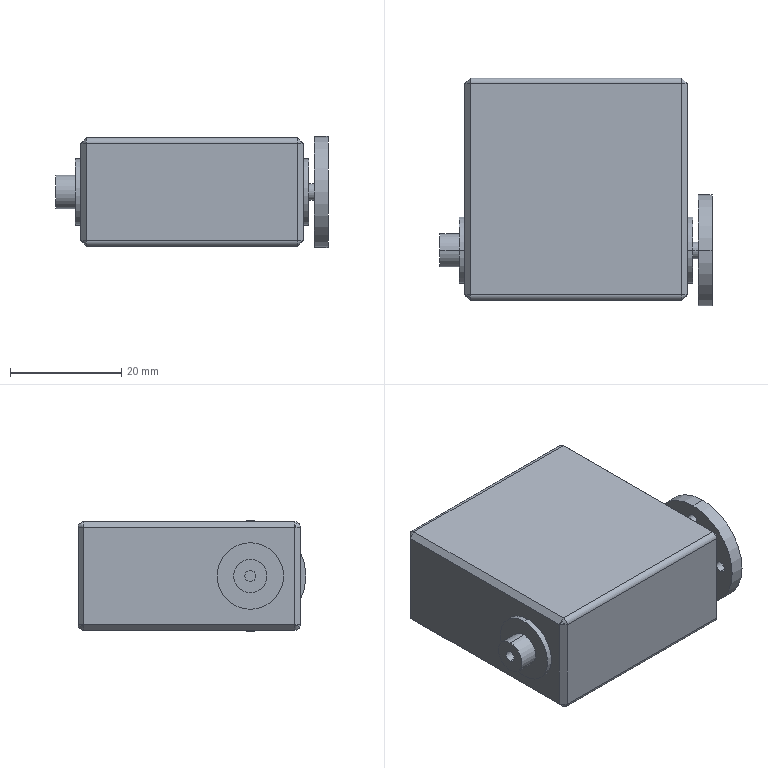Part | SolidWorks | features ICE 7, Chamfer 1, Extrusion 1, Fillet 1 | 1 solid | 52 faces | box 49 x 41 x 20 mm | volume 32126 mm3 | cylinder 24 | plane 20 | cone 8 | commonest cylinder face diameters 2 x14 12 x4 3 x2 6 x2 20 x2
STEP:
#1=CARTESIAN_POINT('',(42.,16.,8.75));
#2=VERTEX_POINT('',#1);
#3=CARTESIAN_POINT('',(42.,16.,10.75));
#4=VERTEX_POINT('',#3);
#5=CARTESIAN_POINT('',(42.,16.,9.75));
#6=DIRECTION('',(-1.,0.,0.));
#7=DIRECTION('',(0.,0.,-1.));
#8=AXIS2_PLACEMENT_3D('',#5,#6,#7);
#9=CIRCLE('',#8,1.);
#10=EDGE_CURVE('',#2,#4,#9,.T.);
#11=ORIENTED_EDGE('',*,*,#10,.T.);
#12=CARTESIAN_POINT('',(44.5,16.,10.75));
#13=VERTEX_POINT('',#12);
#14=CARTESIAN_POINT('',(-4.501,16.,10.75));
#15=DIRECTION('',(1.,0.,0.));
#16=VECTOR('',#15,1000.);
#17=LINE('',#14,#16);
#18=EDGE_CURVE('',#4,#13,#17,.T.);
#19=ORIENTED_EDGE('',*,*,#18,.T.);
#20=CARTESIAN_POINT('',(44.5,16.,8.75));
#21=VERTEX_POINT('',#20);
#22=CARTESIAN_POINT('',(44.5,16.,9.75));
#23=DIRECTION('',(1.,0.,0.));
#24=DIRECTION('',(0.,0.,-1.));
#25=AXIS2_PLACEMENT_3D('',#22,#23,#24);
#26=CIRCLE('',#25,1.);
#27=EDGE_CURVE('',#13,#21,#26,.T.);
#28=ORIENTED_EDGE('',*,*,#27,.T.);
#29=CARTESIAN_POINT('',(-4.501,16.,8.75));
#30=DIRECTION('',(1.,0.,0.));
#31=VECTOR('',#30,1000.);
#32=LINE('',#29,#31);
#33=EDGE_CURVE('',#2,#21,#32,.T.);
#34=ORIENTED_EDGE('',*,*,#33,.F.);
#35=EDGE_LOOP('',(#11,#19,#28,#34));
#36=FACE_OUTER_BOUND('',#35,.T.);
#37=CARTESIAN_POINT('',(-4.501,16.,9.75));
#38=DIRECTION('',(1.,0.,0.));
#39=DIRECTION('',(0.,0.,-1.));
#40=AXIS2_PLACEMENT_3D('',#37,#38,#39);
#41=CYLINDRICAL_SURFACE('',#40,1.);
#42=ADVANCED_FACE('',(#36),#41,.F.);
#43=CARTESIAN_POINT('',(42.,9.,15.75));
#44=VERTEX_POINT('',#43);
#45=CARTESIAN_POINT('',(42.,9.,17.75));
#46=VERTEX_POINT('',#45);
#47=CARTESIAN_POINT('',(42.,9.,16.75));
#48=DIRECTION('',(-1.,0.,0.));
#49=DIRECTION('',(0.,0.,-1.));
#50=AXIS2_PLACEMENT_3D('',#47,#48,#49);
#51=CIRCLE('',#50,1.);
#52=EDGE_CURVE('',#44,#46,#51,.T.);
#53=ORIENTED_EDGE('',*,*,#52,.T.);
#54=CARTESIAN_POINT('',(44.5,9.,17.75));
#55=VERTEX_POINT('',#54);
#56=CARTESIAN_POINT('',(-4.501,9.,17.75));
#57=DIRECTION('',(1.,0.,0.));
#58=VECTOR('',#57,1000.);
#59=LINE('',#56,#58);
#60=EDGE_CURVE('',#46,#55,#59,.T.);
#61=ORIENTED_EDGE('',*,*,#60,.T.);
#62=CARTESIAN_POINT('',(44.5,9.,15.75));
#63=VERTEX_POINT('',#62);
#64=CARTESIAN_POINT('',(44.5,9.,16.75));
#65=DIRECTION('',(1.,0.,0.));
#66=DIRECTION('',(0.,0.,-1.));
#67=AXIS2_PLACEMENT_3D('',#64,#65,#66);
#68=CIRCLE('',#67,1.);
#69=EDGE_CURVE('',#55,#63,#68,.T.);
#70=ORIENTED_EDGE('',*,*,#69,.T.);
#71=CARTESIAN_POINT('',(-4.501,9.,15.75));
#72=DIRECTION('',(1.,0.,0.));
#73=VECTOR('',#72,1000.);
#74=LINE('',#71,#73);
#75=EDGE_CURVE('',#44,#63,#74,.T.);
#76=ORIENTED_EDGE('',*,*,#75,.F.);
#77=EDGE_LOOP('',(#53,#61,#70,#76));
#78=FACE_OUTER_BOUND('',#77,.T.);
#79=CARTESIAN_POINT('',(-4.501,9.,16.75));
#80=DIRECTION('',(1.,0.,0.));
#81=DIRECTION('',(0.,0.,-1.));
#82=AXIS2_PLACEMENT_3D('',#79,#80,#81);
#83=CYLINDRICAL_SURFACE('',#82,1.);
#84=ADVANCED_FACE('',(#78),#83,.F.);
#85=CARTESIAN_POINT('',(42.,9.,1.75));
#86=VERTEX_POINT('',#85);
#87=CARTESIAN_POINT('',(42.,9.,3.75));
#88=VERTEX_POINT('',#87);
#89=CARTESIAN_POINT('',(42.,9.,2.75));
#90=DIRECTION('',(-1.,0.,0.));
#91=DIRECTION('',(0.,0.,-1.));
#92=AXIS2_PLACEMENT_3D('',#89,#90,#91);
#93=CIRCLE('',#92,1.);
#94=EDGE_CURVE('',#86,#88,#93,.T.);
#95=ORIENTED_EDGE('',*,*,#94,.T.);
#96=CARTESIAN_POINT('',(44.5,9.,3.75));
#97=VERTEX_POINT('',#96);
#98=CARTESIAN_POINT('',(-4.501,9.,3.75));
#99=DIRECTION('',(1.,0.,0.));
#100=VECTOR('',#99,1000.);
#101=LINE('',#98,#100);
#102=EDGE_CURVE('',#88,#97,#101,.T.);
#103=ORIENTED_EDGE('',*,*,#102,.T.);
#104=CARTESIAN_POINT('',(44.5,9.,1.75));
#105=VERTEX_POINT('',#104);
#106=CARTESIAN_POINT('',(44.5,9.,2.75));
#107=DIRECTION('',(1.,0.,0.));
#108=DIRECTION('',(0.,0.,-1.));
#109=AXIS2_PLACEMENT_3D('',#106,#107,#108);
#110=CIRCLE('',#109,1.);
#111=EDGE_CURVE('',#97,#105,#110,.T.);
#112=ORIENTED_EDGE('',*,*,#111,.T.);
#113=CARTESIAN_POINT('',(-4.501,9.,1.75));
#114=DIRECTION('',(1.,0.,0.));
#115=VECTOR('',#114,1000.);
#116=LINE('',#113,#115);
#117=EDGE_CURVE('',#86,#105,#116,.T.);
#118=ORIENTED_EDGE('',*,*,#117,.F.);
#119=EDGE_LOOP('',(#95,#103,#112,#118));
#120=FACE_OUTER_BOUND('',#119,.T.);
#121=CARTESIAN_POINT('',(-4.501,9.,2.75));
#122=DIRECTION('',(1.,0.,0.));
#123=DIRECTION('',(0.,0.,-1.));
#124=AXIS2_PLACEMENT_3D('',#121,#122,#123);
#125=CYLINDRICAL_SURFACE('',#124,1.);
#126=ADVANCED_FACE('',(#120),#125,.F.);
#127=CARTESIAN_POINT('',(42.,2.,8.75));
#128=VERTEX_POINT('',#127);
#129=CARTESIAN_POINT('',(42.,2.,10.75));
#130=VERTEX_POINT('',#129);
#131=CARTESIAN_POINT('',(42.,2.,9.75));
#132=DIRECTION('',(-1.,0.,0.));
#133=DIRECTION('',(0.,0.,-1.));
#134=AXIS2_PLACEMENT_3D('',#131,#132,#133);
#135=CIRCLE('',#134,1.);
#136=EDGE_CURVE('',#128,#130,#135,.T.);
#137=ORIENTED_EDGE('',*,*,#136,.T.);
#138=CARTESIAN_POINT('',(44.5,2.,10.75));
#139=VERTEX_POINT('',#138);
#140=CARTESIAN_POINT('',(-4.501,2.,10.75));
#141=DIRECTION('',(1.,0.,0.));
#142=VECTOR('',#141,1000.);
#143=LINE('',#140,#142);
#144=EDGE_CURVE('',#130,#139,#143,.T.);
#145=ORIENTED_EDGE('',*,*,#144,.T.);
#146=CARTESIAN_POINT('',(44.5,2.,8.75));
#147=VERTEX_POINT('',#146);
#148=CARTESIAN_POINT('',(44.5,2.,9.75));
#149=DIRECTION('',(1.,0.,0.));
#150=DIRECTION('',(0.,0.,-1.));
#151=AXIS2_PLACEMENT_3D('',#148,#149,#150);
#152=CIRCLE('',#151,1.);
#153=EDGE_CURVE('',#139,#147,#152,.T.);
#154=ORIENTED_EDGE('',*,*,#153,.T.);
#155=CARTESIAN_POINT('',(-4.501,2.,8.75));
#156=DIRECTION('',(1.,0.,0.));
#157=VECTOR('',#156,1000.);
#158=LINE('',#155,#157);
#159=EDGE_CURVE('',#128,#147,#158,.T.);
#160=ORIENTED_EDGE('',*,*,#159,.F.);
#161=EDGE_LOOP('',(#137,#145,#154,#160));
#162=FACE_OUTER_BOUND('',#161,.T.);
#163=CARTESIAN_POINT('',(-4.501,2.,9.75));
#164=DIRECTION('',(1.,0.,0.));
#165=DIRECTION('',(0.,0.,-1.));
#166=AXIS2_PLACEMENT_3D('',#163,#164,#165);
#167=CYLINDRICAL_SURFACE('',#166,1.);
#168=ADVANCED_FACE('',(#162),#167,.F.);
#169=CARTESIAN_POINT('',(44.5,9.,-0.25));
#170=VERTEX_POINT('',#169);
#171=CARTESIAN_POINT('',(44.5,9.,19.75));
#172=VERTEX_POINT('',#171);
#173=CARTESIAN_POINT('',(44.5,9.,9.75));
#174=DIRECTION('',(1.,0.,0.));
#175=DIRECTION('',(0.,0.,-1.));
#176=AXIS2_PLACEMENT_3D('',#173,#174,#175);
#177=CIRCLE('',#176,10.);
#178=EDGE_CURVE('',#170,#172,#177,.T.);
#179=ORIENTED_EDGE('',*,*,#178,.F.);
#180=CARTESIAN_POINT('',(42.,9.,-0.25));
#181=VERTEX_POINT('',#180);
#182=CARTESIAN_POINT('',(44.5,9.,-0.25));
#183=DIRECTION('',(-1.,0.,0.));
#184=VECTOR('',#183,1000.);
#185=LINE('',#182,#184);
#186=EDGE_CURVE('',#170,#181,#185,.T.);
#187=ORIENTED_EDGE('',*,*,#186,.T.);
#188=CARTESIAN_POINT('',(42.,9.,19.75));
#189=VERTEX_POINT('',#188);
#190=CARTESIAN_POINT('',(42.,9.,9.75));
#191=DIRECTION('',(1.,0.,0.));
#192=DIRECTION('',(0.,0.,-1.));
#193=AXIS2_PLACEMENT_3D('',#190,#191,#192);
#194=CIRCLE('',#193,10.);
#195=EDGE_CURVE('',#181,#189,#194,.T.);
#196=ORIENTED_EDGE('',*,*,#195,.T.);
#197=CARTESIAN_POINT('',(44.5,9.,19.75));
#198=DIRECTION('',(-1.,0.,0.));
#199=VECTOR('',#198,1000.);
#200=LINE('',#197,#199);
#201=EDGE_CURVE('',#172,#189,#200,.T.);
#202=ORIENTED_EDGE('',*,*,#201,.F.);
#203=EDGE_LOOP('',(#179,#187,#196,#202));
#204=FACE_OUTER_BOUND('',#203,.T.);
#205=CARTESIAN_POINT('',(44.5,9.,9.75));
#206=DIRECTION('',(-1.,0.,0.));
#207=DIRECTION('',(0.,0.,1.));
#208=AXIS2_PLACEMENT_3D('',#205,#206,#207);
#209=CYLINDRICAL_SURFACE('',#208,10.);
#210=ADVANCED_FACE('',(#204),#209,.T.);
#211=CARTESIAN_POINT('',(42.,9.,8.25));
#212=VERTEX_POINT('',#211);
#213=CARTESIAN_POINT('',(42.,9.,11.25));
#214=VERTEX_POINT('',#213);
#215=CARTESIAN_POINT('',(42.,9.,9.75));
#216=DIRECTION('',(1.,0.,0.));
#217=DIRECTION('',(0.,0.,-1.));
#218=AXIS2_PLACEMENT_3D('',#215,#216,#217);
#219=CIRCLE('',#218,1.5);
#220=EDGE_CURVE('',#212,#214,#219,.T.);
#221=ORIENTED_EDGE('',*,*,#220,.F.);
#222=CARTESIAN_POINT('',(41.,9.,8.25));
#223=VERTEX_POINT('',#222);
#224=CARTESIAN_POINT('',(42.,9.,8.25));
#225=DIRECTION('',(-1.,0.,0.));
#226=VECTOR('',#225,1000.);
#227=LINE('',#224,#226);
#228=EDGE_CURVE('',#212,#223,#227,.T.);
#229=ORIENTED_EDGE('',*,*,#228,.T.);
#230=CARTESIAN_POINT('',(41.,9.,11.25));
#231=VERTEX_POINT('',#230);
#232=CARTESIAN_POINT('',(41.,9.,9.75));
#233=DIRECTION('',(1.,0.,0.));
#234=DIRECTION('',(0.,0.,-1.));
#235=AXIS2_PLACEMENT_3D('',#232,#233,#234);
#236=CIRCLE('',#235,1.5);
#237=EDGE_CURVE('',#223,#231,#236,.T.);
#238=ORIENTED_EDGE('',*,*,#237,.T.);
#239=CARTESIAN_POINT('',(42.,9.,11.25));
#240=DIRECTION('',(-1.,0.,0.));
#241=VECTOR('',#240,1000.);
#242=LINE('',#239,#241);
#243=EDGE_CURVE('',#214,#231,#242,.T.);
#244=ORIENTED_EDGE('',*,*,#243,.F.);
#245=EDGE_LOOP('',(#221,#229,#238,#244));
#246=FACE_OUTER_BOUND('',#245,.T.);
#247=CARTESIAN_POINT('',(42.,9.,9.75));
#248=DIRECTION('',(-1.,0.,0.));
#249=DIRECTION('',(0.,0.,1.));
#250=AXIS2_PLACEMENT_3D('',#247,#248,#249);
#251=CYLINDRICAL_SURFACE('',#250,1.5);
#252=ADVANCED_FACE('',(#246),#251,.T.);
#253=CARTESIAN_POINT('',(41.,9.,3.75));
#254=VERTEX_POINT('',#253);
#255=CARTESIAN_POINT('',(41.,9.,15.75));
#256=VERTEX_POINT('',#255);
#257=CARTESIAN_POINT('',(41.,9.,9.75));
#258=DIRECTION('',(1.,0.,0.));
#259=DIRECTION('',(0.,0.,-1.));
#260=AXIS2_PLACEMENT_3D('',#257,#258,#259);
#261=CIRCLE('',#260,6.);
#262=EDGE_CURVE('',#254,#256,#261,.T.);
#263=ORIENTED_EDGE('',*,*,#262,.F.);
#264=CARTESIAN_POINT('',(40.,9.,3.75));
#265=VERTEX_POINT('',#264);
#266=CARTESIAN_POINT('',(41.,9.,3.75));
#267=DIRECTION('',(-1.,0.,0.));
#268=VECTOR('',#267,1000.);
#269=LINE('',#266,#268);
#270=EDGE_CURVE('',#254,#265,#269,.T.);
#271=ORIENTED_EDGE('',*,*,#270,.T.);
#272=CARTESIAN_POINT('',(40.,9.,15.75));
#273=VERTEX_POINT('',#272);
#274=CARTESIAN_POINT('',(40.,9.,9.75));
#275=DIRECTION('',(1.,0.,0.));
#276=DIRECTION('',(0.,0.,1.));
#277=AXIS2_PLACEMENT_3D('',#274,#275,#276);
#278=CIRCLE('',#277,6.);
#279=EDGE_CURVE('',#265,#273,#278,.T.);
#280=ORIENTED_EDGE('',*,*,#279,.T.);
#281=CARTESIAN_POINT('',(41.,9.,15.75));
#282=DIRECTION('',(-1.,0.,0.));
#283=VECTOR('',#282,1000.);
#284=LINE('',#281,#283);
#285=EDGE_CURVE('',#256,#273,#284,.T.);
#286=ORIENTED_EDGE('',*,*,#285,.F.);
#287=EDGE_LOOP('',(#263,#271,#280,#286));
#288=FACE_OUTER_BOUND('',#287,.T.);
#289=CARTESIAN_POINT('',(41.,9.,9.75));
#290=DIRECTION('',(-1.,0.,0.));
#291=DIRECTION('',(0.,0.,1.));
#292=AXIS2_PLACEMENT_3D('',#289,#290,#291);
#293=CYLINDRICAL_SURFACE('',#292,6.);
#294=ADVANCED_FACE('',(#288),#293,.T.);
#295=CARTESIAN_POINT('',(-1.,9.,8.75));
#296=VERTEX_POINT('',#295);
#297=CARTESIAN_POINT('',(-1.,9.,10.75));
#298=VERTEX_POINT('',#297);
#299=CARTESIAN_POINT('',(-1.,9.,9.75));
#300=DIRECTION('',(-1.,0.,0.));
#301=DIRECTION('',(0.,0.,1.));
#302=AXIS2_PLACEMENT_3D('',#299,#300,#301);
#303=CIRCLE('',#302,1.);
#304=EDGE_CURVE('',#296,#298,#303,.T.);
#305=ORIENTED_EDGE('',*,*,#304,.F.);
#306=CARTESIAN_POINT('',(-4.5,9.,8.75));
#307=VERTEX_POINT('',#306);
#308=CARTESIAN_POINT('',(-1.,9.,8.75));
#309=DIRECTION('',(-1.,0.,0.));
#310=VECTOR('',#309,1000.);
#311=LINE('',#308,#310);
#312=EDGE_CURVE('',#296,#307,#311,.T.);
#313=ORIENTED_EDGE('',*,*,#312,.T.);
#314=CARTESIAN_POINT('',(-4.5,9.,10.75));
#315=VERTEX_POINT('',#314);
#316=CARTESIAN_POINT('',(-4.5,9.,9.75));
#317=DIRECTION('',(-1.,0.,0.));
#318=DIRECTION('',(0.,0.,1.));
#319=AXIS2_PLACEMENT_3D('',#316,#317,#318);
#320=CIRCLE('',#319,1.);
#321=EDGE_CURVE('',#307,#315,#320,.T.);
#322=ORIENTED_EDGE('',*,*,#321,.T.);
#323=CARTESIAN_POINT('',(-1.,9.,10.75));
#324=DIRECTION('',(-1.,0.,0.));
#325=VECTOR('',#324,1000.);
#326=LINE('',#323,#325);
#327=EDGE_CURVE('',#298,#315,#326,.T.);
#328=ORIENTED_EDGE('',*,*,#327,.F.);
#329=EDGE_LOOP('',(#305,#313,#322,#328));
#330=FACE_OUTER_BOUND('',#329,.T.);
#331=CARTESIAN_POINT('',(-1.,9.,9.75));
#332=DIRECTION('',(-1.,0.,0.));
#333=DIRECTION('',(0.,0.,1.));
#334=AXIS2_PLACEMENT_3D('',#331,#332,#333);
#335=CYLINDRICAL_SURFACE('',#334,1.);
#336=ADVANCED_FACE('',(#330),#335,.F.);
#337=CARTESIAN_POINT('',(-4.5,9.,12.75));
#338=VERTEX_POINT('',#337);
#339=CARTESIAN_POINT('',(-4.5,9.,6.75));
#340=VERTEX_POINT('',#339);
#341=CARTESIAN_POINT('',(-4.5,9.,9.75));
#342=DIRECTION('',(-1.,0.,0.));
#343=DIRECTION('',(0.,0.,1.));
#344=AXIS2_PLACEMENT_3D('',#341,#342,#343);
#345=CIRCLE('',#344,3.);
#346=EDGE_CURVE('',#338,#340,#345,.T.);
#347=ORIENTED_EDGE('',*,*,#346,.F.);
#348=CARTESIAN_POINT('',(-1.,9.,12.75));
#349=VERTEX_POINT('',#348);
#350=CARTESIAN_POINT('',(-4.5,9.,12.75));
#351=DIRECTION('',(1.,0.,0.));
#352=VECTOR('',#351,1000.);
#353=LINE('',#350,#352);
#354=EDGE_CURVE('',#338,#349,#353,.T.);
#355=ORIENTED_EDGE('',*,*,#354,.T.);
#356=CARTESIAN_POINT('',(-1.,9.,6.75));
#357=VERTEX_POINT('',#356);
#358=CARTESIAN_POINT('',(-1.,9.,9.75));
#359=DIRECTION('',(-1.,0.,0.));
#360=DIRECTION('',(0.,0.,1.));
#361=AXIS2_PLACEMENT_3D('',#358,#359,#360);
#362=CIRCLE('',#361,3.);
#363=EDGE_CURVE('',#349,#357,#362,.T.);
#364=ORIENTED_EDGE('',*,*,#363,.T.);
#365=CARTESIAN_POINT('',(-4.5,9.,6.75));
#366=DIRECTION('',(1.,0.,0.));
#367=VECTOR('',#366,1000.);
#368=LINE('',#365,#367);
#369=EDGE_CURVE('',#340,#357,#368,.T.);
#370=ORIENTED_EDGE('',*,*,#369,.F.);
#371=EDGE_LOOP('',(#347,#355,#364,#370));
#372=FACE_OUTER_BOUND('',#371,.T.);
#373=CARTESIAN_POINT('',(-4.5,9.,9.75));
#374=DIRECTION('',(1.,0.,0.));
#375=DIRECTION('',(0.,0.,-1.));
#376=AXIS2_PLACEMENT_3D('',#373,#374,#375);
#377=CYLINDRICAL_SURFACE('',#376,3.);
#378=ADVANCED_FACE('',(#372),#377,.T.);
#379=CARTESIAN_POINT('',(-1.,9.,15.75));
#380=VERTEX_POINT('',#379);
#381=CARTESIAN_POINT('',(-1.,9.,3.75));
#382=VERTEX_POINT('',#381);
#383=CARTESIAN_POINT('',(-1.,9.,9.75));
#384=DIRECTION('',(-1.,0.,0.));
#385=DIRECTION('',(0.,0.,1.));
#386=AXIS2_PLACEMENT_3D('',#383,#384,#385);
#387=CIRCLE('',#386,6.);
#388=EDGE_CURVE('',#380,#382,#387,.T.);
#389=ORIENTED_EDGE('',*,*,#388,.F.);
#390=CARTESIAN_POINT('',(0.,9.,15.75));
#391=VERTEX_POINT('',#390);
#392=CARTESIAN_POINT('',(-1.,9.,15.75));
#393=DIRECTION('',(1.,0.,0.));
#394=VECTOR('',#393,1000.);
#395=LINE('',#392,#394);
#396=EDGE_CURVE('',#380,#391,#395,.T.);
#397=ORIENTED_EDGE('',*,*,#396,.T.);
#398=CARTESIAN_POINT('',(0.,9.,3.75));
#399=VERTEX_POINT('',#398);
#400=CARTESIAN_POINT('',(0.,9.,9.75));
#401=DIRECTION('',(-1.,0.,0.));
#402=DIRECTION('',(0.,0.,-1.));
#403=AXIS2_PLACEMENT_3D('',#400,#401,#402);
#404=CIRCLE('',#403,6.);
#405=EDGE_CURVE('',#391,#399,#404,.T.);
#406=ORIENTED_EDGE('',*,*,#405,.T.);
#407=CARTESIAN_POINT('',(-1.,9.,3.75));
#408=DIRECTION('',(1.,0.,0.));
#409=VECTOR('',#408,1000.);
#410=LINE('',#407,#409);
#411=EDGE_CURVE('',#382,#399,#410,.T.);
#412=ORIENTED_EDGE('',*,*,#411,.F.);
#413=EDGE_LOOP('',(#389,#397,#406,#412));
#414=FACE_OUTER_BOUND('',#413,.T.);
#415=CARTESIAN_POINT('',(-1.,9.,9.75));
#416=DIRECTION('',(1.,0.,0.));
#417=DIRECTION('',(0.,0.,-1.));
#418=AXIS2_PLACEMENT_3D('',#415,#416,#417);
#419=CYLINDRICAL_SURFACE('',#418,6.);
#420=ADVANCED_FACE('',(#414),#419,.T.);
#421=CARTESIAN_POINT('',(0.,9.,9.75));
#422=DIRECTION('',(-1.,0.,0.));
#423=DIRECTION('',(0.,0.,-1.));
#424=AXIS2_PLACEMENT_3D('',#421,#422,#423);
#425=CIRCLE('',#424,6.);
#426=EDGE_CURVE('',#399,#391,#425,.T.);
#427=ORIENTED_EDGE('',*,*,#426,.F.);
#428=ORIENTED_EDGE('',*,*,#405,.F.);
#429=EDGE_LOOP('',(#427,#428));
#430=FACE_BOUND('',#429,.T.);
#431=CARTESIAN_POINT('',(0.,39.,18.5));
#432=VERTEX_POINT('',#431);
#433=CARTESIAN_POINT('',(0.,39.,1.));
#434=VERTEX_POINT('',#433);
#435=CARTESIAN_POINT('',(0.,39.,19.5));
#436=DIRECTION('',(0.,0.,-1.));
#437=VECTOR('',#436,1000.);
#438=LINE('',#435,#437);
#439=EDGE_CURVE('',#432,#434,#438,.T.);
#440=ORIENTED_EDGE('',*,*,#439,.T.);
#441=CARTESIAN_POINT('',(0.,1.,1.));
#442=VERTEX_POINT('',#441);
#443=CARTESIAN_POINT('',(0.,1.,1.));
#444=DIRECTION('',(0.,-1.,0.));
#445=VECTOR('',#444,1000.);
#446=LINE('',#443,#445);
#447=EDGE_CURVE('',#434,#442,#446,.T.);
#448=ORIENTED_EDGE('',*,*,#447,.T.);
#449=CARTESIAN_POINT('',(0.,1.,18.5));
#450=VERTEX_POINT('',#449);
#451=CARTESIAN_POINT('',(0.,1.,19.5));
#452=DIRECTION('',(0.,0.,1.));
#453=VECTOR('',#452,1000.);
#454=LINE('',#451,#453);
#455=EDGE_CURVE('',#442,#450,#454,.T.);
#456=ORIENTED_EDGE('',*,*,#455,.T.);
#457=CARTESIAN_POINT('',(0.,0.,18.5));
#458=DIRECTION('',(0.,1.,0.));
#459=VECTOR('',#458,1000.);
#460=LINE('',#457,#459);
#461=EDGE_CURVE('',#450,#432,#460,.T.);
#462=ORIENTED_EDGE('',*,*,#461,.T.);
#463=EDGE_LOOP('',(#440,#448,#456,#462));
#464=FACE_OUTER_BOUND('',#463,.T.);
#465=CARTESIAN_POINT('',(0.,0.,19.5));
#466=DIRECTION('',(1.,0.,0.));
#467=DIRECTION('',(0.,0.,-1.));
#468=AXIS2_PLACEMENT_3D('',#465,#466,#467);
#469=PLANE('',#468);
#470=ADVANCED_FACE('',(#430,#464),#469,.F.);
#471=CARTESIAN_POINT('',(1.,0.,1.));
#472=VERTEX_POINT('',#471);
#473=CARTESIAN_POINT('',(39.,0.,1.));
#474=VERTEX_POINT('',#473);
#475=CARTESIAN_POINT('',(40.,0.,1.));
#476=DIRECTION('',(1.,0.,0.));
#477=VECTOR('',#476,1000.);
#478=LINE('',#475,#477);
#479=EDGE_CURVE('',#472,#474,#478,.T.);
#480=ORIENTED_EDGE('',*,*,#479,.T.);
#481=CARTESIAN_POINT('',(39.,0.,18.5));
#482=VERTEX_POINT('',#481);
#483=CARTESIAN_POINT('',(39.,0.,19.5));
#484=DIRECTION('',(0.,0.,1.));
#485=VECTOR('',#484,1000.);
#486=LINE('',#483,#485);
#487=EDGE_CURVE('',#474,#482,#486,.T.);
#488=ORIENTED_EDGE('',*,*,#487,.T.);
#489=CARTESIAN_POINT('',(1.,0.,18.5));
#490=VERTEX_POINT('',#489);
#491=CARTESIAN_POINT('',(0.,0.,18.5));
#492=DIRECTION('',(-1.,0.,0.));
#493=VECTOR('',#492,1000.);
#494=LINE('',#491,#493);
#495=EDGE_CURVE('',#482,#490,#494,.T.);
#496=ORIENTED_EDGE('',*,*,#495,.T.);
#497=CARTESIAN_POINT('',(1.,0.,19.5));
#498=DIRECTION('',(0.,0.,-1.));
#499=VECTOR('',#498,1000.);
#500=LINE('',#497,#499);
#501=EDGE_CURVE('',#490,#472,#500,.T.);
#502=ORIENTED_EDGE('',*,*,#501,.T.);
#503=EDGE_LOOP('',(#480,#488,#496,#502));
#504=FACE_OUTER_BOUND('',#503,.T.);
#505=CARTESIAN_POINT('',(0.,0.,19.5));
#506=DIRECTION('',(0.,1.,0.));
#507=DIRECTION('',(0.,0.,1.));
#508=AXIS2_PLACEMENT_3D('',#505,#506,#507);
#509=PLANE('',#508);
#510=ADVANCED_FACE('',(#504),#509,.F.);
#511=CARTESIAN_POINT('',(40.,9.,9.75));
#512=DIRECTION('',(1.,0.,0.));
#513=DIRECTION('',(0.,0.,1.));
#514=AXIS2_PLACEMENT_3D('',#511,#512,#513);
#515=CIRCLE('',#514,6.);
#516=EDGE_CURVE('',#273,#265,#515,.T.);
#517=ORIENTED_EDGE('',*,*,#516,.F.);
#518=ORIENTED_EDGE('',*,*,#279,.F.);
#519=EDGE_LOOP('',(#517,#518));
#520=FACE_BOUND('',#519,.T.);
#521=CARTESIAN_POINT('',(40.,1.,18.5));
#522=VERTEX_POINT('',#521);
#523=CARTESIAN_POINT('',(40.,1.,1.));
#524=VERTEX_POINT('',#523);
#525=CARTESIAN_POINT('',(40.,1.,19.5));
#526=DIRECTION('',(0.,0.,-1.));
#527=VECTOR('',#526,1000.);
#528=LINE('',#525,#527);
#529=EDGE_CURVE('',#522,#524,#528,.T.);
#530=ORIENTED_EDGE('',*,*,#529,.T.);
#531=CARTESIAN_POINT('',(40.,39.,1.));
#532=VERTEX_POINT('',#531);
#533=CARTESIAN_POINT('',(40.,39.,1.));
#534=DIRECTION('',(0.,1.,0.));
#535=VECTOR('',#534,1000.);
#536=LINE('',#533,#535);
#537=EDGE_CURVE('',#524,#532,#536,.T.);
#538=ORIENTED_EDGE('',*,*,#537,.T.);
#539=CARTESIAN_POINT('',(40.,39.,18.5));
#540=VERTEX_POINT('',#539);
#541=CARTESIAN_POINT('',(40.,39.,19.5));
#542=DIRECTION('',(0.,0.,1.));
#543=VECTOR('',#542,1000.);
#544=LINE('',#541,#543);
#545=EDGE_CURVE('',#532,#540,#544,.T.);
#546=ORIENTED_EDGE('',*,*,#545,.T.);
#547=CARTESIAN_POINT('',(40.,0.,18.5));
#548=DIRECTION('',(0.,-1.,0.));
#549=VECTOR('',#548,1000.);
#550=LINE('',#547,#549);
#551=EDGE_CURVE('',#540,#522,#550,.T.);
#552=ORIENTED_EDGE('',*,*,#551,.T.);
#553=EDGE_LOOP('',(#530,#538,#546,#552));
#554=FACE_OUTER_BOUND('',#553,.T.);
#555=CARTESIAN_POINT('',(40.,0.,19.5));
#556=DIRECTION('',(-1.,0.,0.));
#557=DIRECTION('',(0.,0.,1.));
#558=AXIS2_PLACEMENT_3D('',#555,#556,#557);
#559=PLANE('',#558);
#560=ADVANCED_FACE('',(#520,#554),#559,.F.);
#561=CARTESIAN_POINT('',(1.,40.,18.5));
#562=VERTEX_POINT('',#561);
#563=CARTESIAN_POINT('',(39.,40.,18.5));
#564=VERTEX_POINT('',#563);
#565=CARTESIAN_POINT('',(0.,40.,18.5));
#566=DIRECTION('',(1.,0.,0.));
#567=VECTOR('',#566,1000.);
#568=LINE('',#565,#567);
#569=EDGE_CURVE('',#562,#564,#568,.T.);
#570=ORIENTED_EDGE('',*,*,#569,.T.);
#571=CARTESIAN_POINT('',(39.,40.,1.));
#572=VERTEX_POINT('',#571);
#573=CARTESIAN_POINT('',(39.,40.,19.5));
#574=DIRECTION('',(0.,0.,-1.));
#575=VECTOR('',#574,1000.);
#576=LINE('',#573,#575);
#577=EDGE_CURVE('',#564,#572,#576,.T.);
#578=ORIENTED_EDGE('',*,*,#577,.T.);
#579=CARTESIAN_POINT('',(1.,40.,1.));
#580=VERTEX_POINT('',#579);
#581=CARTESIAN_POINT('',(0.,40.,1.));
#582=DIRECTION('',(-1.,0.,0.));
#583=VECTOR('',#582,1000.);
#584=LINE('',#581,#583);
#585=EDGE_CURVE('',#572,#580,#584,.T.);
#586=ORIENTED_EDGE('',*,*,#585,.T.);
#587=CARTESIAN_POINT('',(1.,40.,19.5));
#588=DIRECTION('',(0.,0.,1.));
#589=VECTOR('',#588,1000.);
#590=LINE('',#587,#589);
#591=EDGE_CURVE('',#580,#562,#590,.T.);
#592=ORIENTED_EDGE('',*,*,#591,.T.);
#593=EDGE_LOOP('',(#570,#578,#586,#592));
#594=FACE_OUTER_BOUND('',#593,.T.);
#595=CARTESIAN_POINT('',(0.,40.,19.5));
#596=DIRECTION('',(0.,-1.,0.));
#597=DIRECTION('',(0.,0.,-1.));
#598=AXIS2_PLACEMENT_3D('',#595,#596,#597);
#599=PLANE('',#598);
#600=ADVANCED_FACE('',(#594),#599,.F.);
#601=CARTESIAN_POINT('',(1.,1.,19.5));
#602=VERTEX_POINT('',#601);
#603=CARTESIAN_POINT('',(39.,1.,19.5));
#604=VERTEX_POINT('',#603);
#605=CARTESIAN_POINT('',(0.,1.,19.5));
#606=DIRECTION('',(1.,0.,0.));
#607=VECTOR('',#606,1000.);
#608=LINE('',#605,#607);
#609=EDGE_CURVE('',#602,#604,#608,.T.);
#610=ORIENTED_EDGE('',*,*,#609,.T.);
#611=CARTESIAN_POINT('',(39.,39.,19.5));
#612=VERTEX_POINT('',#611);
#613=CARTESIAN_POINT('',(39.,0.,19.5));
#614=DIRECTION('',(0.,1.,0.));
#615=VECTOR('',#614,1000.);
#616=LINE('',#613,#615);
#617=EDGE_CURVE('',#604,#612,#616,.T.);
#618=ORIENTED_EDGE('',*,*,#617,.T.);
#619=CARTESIAN_POINT('',(1.,39.,19.5));
#620=VERTEX_POINT('',#619);
#621=CARTESIAN_POINT('',(0.,39.,19.5));
#622=DIRECTION('',(-1.,0.,0.));
#623=VECTOR('',#622,1000.);
#624=LINE('',#621,#623);
#625=EDGE_CURVE('',#612,#620,#624,.T.);
#626=ORIENTED_EDGE('',*,*,#625,.T.);
#627=CARTESIAN_POINT('',(1.,0.,19.5));
#628=DIRECTION('',(0.,-1.,0.));
#629=VECTOR('',#628,1000.);
#630=LINE('',#627,#629);
#631=EDGE_CURVE('',#620,#602,#630,.T.);
#632=ORIENTED_EDGE('',*,*,#631,.T.);
#633=EDGE_LOOP('',(#610,#618,#626,#632));
#634=FACE_OUTER_BOUND('',#633,.T.);
#635=CARTESIAN_POINT('',(0.,0.,19.5));
#636=DIRECTION('',(0.,0.,-1.));
#637=DIRECTION('',(-1.,0.,0.));
#638=AXIS2_PLACEMENT_3D('',#635,#636,#637);
#639=PLANE('',#638);
#640=ADVANCED_FACE('',(#634),#639,.F.);
#641=CARTESIAN_POINT('',(1.,39.,0.));
#642=VERTEX_POINT('',#641);
#643=CARTESIAN_POINT('',(39.,39.,0.));
#644=VERTEX_POINT('',#643);
#645=CARTESIAN_POINT('',(40.,39.,0.));
#646=DIRECTION('',(1.,0.,0.));
#647=VECTOR('',#646,1000.);
#648=LINE('',#645,#647);
#649=EDGE_CURVE('',#642,#644,#648,.T.);
#650=ORIENTED_EDGE('',*,*,#649,.T.);
#651=CARTESIAN_POINT('',(39.,1.,0.));
#652=VERTEX_POINT('',#651);
#653=CARTESIAN_POINT('',(39.,1.,0.));
#654=DIRECTION('',(0.,-1.,0.));
#655=VECTOR('',#654,1000.);
#656=LINE('',#653,#655);
#657=EDGE_CURVE('',#644,#652,#656,.T.);
#658=ORIENTED_EDGE('',*,*,#657,.T.);
#659=CARTESIAN_POINT('',(1.,1.,0.));
#660=VERTEX_POINT('',#659);
#661=CARTESIAN_POINT('',(0.,1.,0.));
#662=DIRECTION('',(-1.,0.,0.));
#663=VECTOR('',#662,1000.);
#664=LINE('',#661,#663);
#665=EDGE_CURVE('',#652,#660,#664,.T.);
#666=ORIENTED_EDGE('',*,*,#665,.T.);
#667=CARTESIAN_POINT('',(1.,39.,0.));
#668=DIRECTION('',(0.,1.,0.));
#669=VECTOR('',#668,1000.);
#670=LINE('',#667,#669);
#671=EDGE_CURVE('',#660,#642,#670,.T.);
#672=ORIENTED_EDGE('',*,*,#671,.T.);
#673=EDGE_LOOP('',(#650,#658,#666,#672));
#674=FACE_OUTER_BOUND('',#673,.T.);
#675=CARTESIAN_POINT('',(0.,0.,0.));
#676=DIRECTION('',(0.,0.,-1.));
#677=DIRECTION('',(-1.,0.,0.));
#678=AXIS2_PLACEMENT_3D('',#675,#676,#677);
#679=PLANE('',#678);
#680=ADVANCED_FACE('',(#674),#679,.T.);
#681=ORIENTED_EDGE('',*,*,#665,.F.);
#682=CARTESIAN_POINT('',(39.,1.,1.));
#683=DIRECTION('',(-1.,0.,0.));
#684=DIRECTION('',(0.,0.,1.));
#685=AXIS2_PLACEMENT_3D('',#682,#683,#684);
#686=CIRCLE('',#685,1.);
#687=EDGE_CURVE('',#652,#474,#686,.T.);
#688=ORIENTED_EDGE('',*,*,#687,.T.);
#689=ORIENTED_EDGE('',*,*,#479,.F.);
#690=CARTESIAN_POINT('',(1.,1.,1.));
#691=DIRECTION('',(1.,0.,0.));
#692=DIRECTION('',(0.,0.,-1.));
#693=AXIS2_PLACEMENT_3D('',#690,#691,#692);
#694=CIRCLE('',#693,1.);
#695=EDGE_CURVE('',#472,#660,#694,.T.);
#696=ORIENTED_EDGE('',*,*,#695,.T.);
#697=EDGE_LOOP('',(#681,#688,#689,#696));
#698=FACE_OUTER_BOUND('',#697,.T.);
#699=CARTESIAN_POINT('',(0.,1.,1.));
#700=DIRECTION('',(-1.,0.,0.));
#701=DIRECTION('',(0.,0.,1.));
#702=AXIS2_PLACEMENT_3D('',#699,#700,#701);
#703=CYLINDRICAL_SURFACE('',#702,1.);
#704=ADVANCED_FACE('',(#698),#703,.T.);
#705=ORIENTED_EDGE('',*,*,#495,.F.);
#706=CARTESIAN_POINT('',(39.,1.,18.5));
#707=DIRECTION('',(-1.,0.,0.));
#708=DIRECTION('',(0.,0.,1.));
#709=AXIS2_PLACEMENT_3D('',#706,#707,#708);
#710=CIRCLE('',#709,1.);
#711=EDGE_CURVE('',#482,#604,#710,.T.);
#712=ORIENTED_EDGE('',*,*,#711,.T.);
#713=ORIENTED_EDGE('',*,*,#609,.F.);
#714=CARTESIAN_POINT('',(1.,1.,18.5));
#715=DIRECTION('',(1.,0.,0.));
#716=DIRECTION('',(0.,0.,-1.));
#717=AXIS2_PLACEMENT_3D('',#714,#715,#716);
#718=CIRCLE('',#717,1.);
#719=EDGE_CURVE('',#602,#490,#718,.T.);
#720=ORIENTED_EDGE('',*,*,#719,.T.);
#721=EDGE_LOOP('',(#705,#712,#713,#720));
#722=FACE_OUTER_BOUND('',#721,.T.);
#723=CARTESIAN_POINT('',(0.,1.,18.5));
#724=DIRECTION('',(1.,0.,0.));
#725=DIRECTION('',(0.,0.,-1.));
#726=AXIS2_PLACEMENT_3D('',#723,#724,#725);
#727=CYLINDRICAL_SURFACE('',#726,1.);
#728=ADVANCED_FACE('',(#722),#727,.T.);
#729=ORIENTED_EDGE('',*,*,#585,.F.);
#730=CARTESIAN_POINT('',(39.,39.,1.));
#731=DIRECTION('',(-1.,0.,0.));
#732=DIRECTION('',(0.,0.,1.));
#733=AXIS2_PLACEMENT_3D('',#730,#731,#732);
#734=CIRCLE('',#733,1.);
#735=EDGE_CURVE('',#572,#644,#734,.T.);
#736=ORIENTED_EDGE('',*,*,#735,.T.);
#737=ORIENTED_EDGE('',*,*,#649,.F.);
#738=CARTESIAN_POINT('',(1.,39.,1.));
#739=DIRECTION('',(1.,0.,0.));
#740=DIRECTION('',(0.,0.,-1.));
#741=AXIS2_PLACEMENT_3D('',#738,#739,#740);
#742=CIRCLE('',#741,1.);
#743=EDGE_CURVE('',#642,#580,#742,.T.);
#744=ORIENTED_EDGE('',*,*,#743,.T.);
#745=EDGE_LOOP('',(#729,#736,#737,#744));
#746=FACE_OUTER_BOUND('',#745,.T.);
#747=CARTESIAN_POINT('',(0.,39.,1.));
#748=DIRECTION('',(1.,0.,0.));
#749=DIRECTION('',(0.,0.,-1.));
#750=AXIS2_PLACEMENT_3D('',#747,#748,#749);
#751=CYLINDRICAL_SURFACE('',#750,1.);
#752=ADVANCED_FACE('',(#746),#751,.T.);
#753=ORIENTED_EDGE('',*,*,#625,.F.);
#754=CARTESIAN_POINT('',(39.,39.,18.5));
#755=DIRECTION('',(-1.,0.,0.));
#756=DIRECTION('',(0.,0.,1.));
#757=AXIS2_PLACEMENT_3D('',#754,#755,#756);
#758=CIRCLE('',#757,1.);
#759=EDGE_CURVE('',#612,#564,#758,.T.);
#760=ORIENTED_EDGE('',*,*,#759,.T.);
#761=ORIENTED_EDGE('',*,*,#569,.F.);
#762=CARTESIAN_POINT('',(1.,39.,18.5));
#763=DIRECTION('',(1.,0.,0.));
#764=DIRECTION('',(0.,0.,-1.));
#765=AXIS2_PLACEMENT_3D('',#762,#763,#764);
#766=CIRCLE('',#765,1.);
#767=EDGE_CURVE('',#562,#620,#766,.T.);
#768=ORIENTED_EDGE('',*,*,#767,.T.);
#769=EDGE_LOOP('',(#753,#760,#761,#768));
#770=FACE_OUTER_BOUND('',#769,.T.);
#771=CARTESIAN_POINT('',(0.,39.,18.5));
#772=DIRECTION('',(-1.,0.,0.));
#773=DIRECTION('',(0.,0.,1.));
#774=AXIS2_PLACEMENT_3D('',#771,#772,#773);
#775=CYLINDRICAL_SURFACE('',#774,1.);
#776=ADVANCED_FACE('',(#770),#775,.T.);
#777=CARTESIAN_POINT('',(39.,39.,19.5));
#778=DIRECTION('',(0.7071,0.,-0.7071));
#779=VECTOR('',#778,1000.);
#780=LINE('',#777,#779);
#781=EDGE_CURVE('',#612,#540,#780,.T.);
#782=ORIENTED_EDGE('',*,*,#781,.F.);
#783=ORIENTED_EDGE('',*,*,#617,.F.);
#784=CARTESIAN_POINT('',(40.,1.,18.5));
#785=DIRECTION('',(-0.7071,0.,0.7071));
#786=VECTOR('',#785,1000.);
#787=LINE('',#784,#786);
#788=EDGE_CURVE('',#522,#604,#787,.T.);
#789=ORIENTED_EDGE('',*,*,#788,.F.);
#790=ORIENTED_EDGE('',*,*,#551,.F.);
#791=EDGE_LOOP('',(#782,#783,#789,#790));
#792=FACE_OUTER_BOUND('',#791,.T.);
#793=CARTESIAN_POINT('',(39.,0.,19.5));
#794=DIRECTION('',(-0.7071,0.,-0.7071));
#795=DIRECTION('',(0.,1.,0.));
#796=AXIS2_PLACEMENT_3D('',#793,#794,#795);
#797=PLANE('',#796);
#798=ADVANCED_FACE('',(#792),#797,.F.);
#799=ORIENTED_EDGE('',*,*,#788,.T.);
#800=ORIENTED_EDGE('',*,*,#711,.F.);
#801=CARTESIAN_POINT('',(40.,1.,18.5));
#802=DIRECTION('',(-0.7071,-0.7071,0.));
#803=VECTOR('',#802,1000.);
#804=LINE('',#801,#803);
#805=EDGE_CURVE('',#522,#482,#804,.T.);
#806=ORIENTED_EDGE('',*,*,#805,.F.);
#807=EDGE_LOOP('',(#799,#800,#806));
#808=FACE_OUTER_BOUND('',#807,.T.);
#809=CARTESIAN_POINT('',(39.,1.,18.5));
#810=DIRECTION('',(-1.,0.,0.));
#811=DIRECTION('',(0.,0.,1.));
#812=AXIS2_PLACEMENT_3D('',#809,#810,#811);
#813=CONICAL_SURFACE('',#812,1.,0.7854);
#814=ADVANCED_FACE('',(#808),#813,.T.);
#815=ORIENTED_EDGE('',*,*,#759,.F.);
#816=ORIENTED_EDGE('',*,*,#781,.T.);
#817=CARTESIAN_POINT('',(39.,40.,18.5));
#818=DIRECTION('',(0.7071,-0.7071,0.));
#819=VECTOR('',#818,1000.);
#820=LINE('',#817,#819);
#821=EDGE_CURVE('',#564,#540,#820,.T.);
#822=ORIENTED_EDGE('',*,*,#821,.F.);
#823=EDGE_LOOP('',(#815,#816,#822));
#824=FACE_OUTER_BOUND('',#823,.T.);
#825=CARTESIAN_POINT('',(39.,39.,18.5));
#826=DIRECTION('',(-1.,0.,0.));
#827=DIRECTION('',(0.,0.,1.));
#828=AXIS2_PLACEMENT_3D('',#825,#826,#827);
#829=CONICAL_SURFACE('',#828,1.,0.7854);
#830=ADVANCED_FACE('',(#824),#829,.T.);
#831=ORIENTED_EDGE('',*,*,#805,.T.);
#832=ORIENTED_EDGE('',*,*,#487,.F.);
#833=CARTESIAN_POINT('',(40.,1.,1.));
#834=DIRECTION('',(-0.7071,-0.7071,0.));
#835=VECTOR('',#834,1000.);
#836=LINE('',#833,#835);
#837=EDGE_CURVE('',#524,#474,#836,.T.);
#838=ORIENTED_EDGE('',*,*,#837,.F.);
#839=ORIENTED_EDGE('',*,*,#529,.F.);
#840=EDGE_LOOP('',(#831,#832,#838,#839));
#841=FACE_OUTER_BOUND('',#840,.T.);
#842=CARTESIAN_POINT('',(40.,1.,19.5));
#843=DIRECTION('',(-0.7071,0.7071,0.));
#844=DIRECTION('',(0.,0.,-1.));
#845=AXIS2_PLACEMENT_3D('',#842,#843,#844);
#846=PLANE('',#845);
#847=ADVANCED_FACE('',(#841),#846,.F.);
#848=ORIENTED_EDGE('',*,*,#821,.T.);
#849=ORIENTED_EDGE('',*,*,#545,.F.);
#850=CARTESIAN_POINT('',(39.,40.,1.));
#851=DIRECTION('',(0.7071,-0.7071,0.));
#852=VECTOR('',#851,1000.);
#853=LINE('',#850,#852);
#854=EDGE_CURVE('',#572,#532,#853,.T.);
#855=ORIENTED_EDGE('',*,*,#854,.F.);
#856=ORIENTED_EDGE('',*,*,#577,.F.);
#857=EDGE_LOOP('',(#848,#849,#855,#856));
#858=FACE_OUTER_BOUND('',#857,.T.);
#859=CARTESIAN_POINT('',(39.,40.,19.5));
#860=DIRECTION('',(-0.7071,-0.7071,0.));
#861=DIRECTION('',(0.,0.,-1.));
#862=AXIS2_PLACEMENT_3D('',#859,#860,#861);
#863=PLANE('',#862);
#864=ADVANCED_FACE('',(#858),#863,.F.);
#865=ORIENTED_EDGE('',*,*,#837,.T.);
#866=ORIENTED_EDGE('',*,*,#687,.F.);
#867=CARTESIAN_POINT('',(40.,1.,1.));
#868=DIRECTION('',(-0.7071,0.,-0.7071));
#869=VECTOR('',#868,1000.);
#870=LINE('',#867,#869);
#871=EDGE_CURVE('',#524,#652,#870,.T.);
#872=ORIENTED_EDGE('',*,*,#871,.F.);
#873=EDGE_LOOP('',(#865,#866,#872));
#874=FACE_OUTER_BOUND('',#873,.T.);
#875=CARTESIAN_POINT('',(39.,1.,1.));
#876=DIRECTION('',(-1.,0.,0.));
#877=DIRECTION('',(0.,0.,1.));
#878=AXIS2_PLACEMENT_3D('',#875,#876,#877);
#879=CONICAL_SURFACE('',#878,1.,0.7854);
#880=ADVANCED_FACE('',(#874),#879,.T.);
#881=ORIENTED_EDGE('',*,*,#735,.F.);
#882=ORIENTED_EDGE('',*,*,#854,.T.);
#883=CARTESIAN_POINT('',(39.,39.,0.));
#884=DIRECTION('',(0.7071,0.,0.7071));
#885=VECTOR('',#884,1000.);
#886=LINE('',#883,#885);
#887=EDGE_CURVE('',#644,#532,#886,.T.);
#888=ORIENTED_EDGE('',*,*,#887,.F.);
#889=EDGE_LOOP('',(#881,#882,#888));
#890=FACE_OUTER_BOUND('',#889,.T.);
#891=CARTESIAN_POINT('',(39.,39.,1.));
#892=DIRECTION('',(-1.,0.,0.));
#893=DIRECTION('',(0.,0.,1.));
#894=AXIS2_PLACEMENT_3D('',#891,#892,#893);
#895=CONICAL_SURFACE('',#894,1.,0.7854);
#896=ADVANCED_FACE('',(#890),#895,.T.);
#897=ORIENTED_EDGE('',*,*,#871,.T.);
#898=ORIENTED_EDGE('',*,*,#657,.F.);
#899=ORIENTED_EDGE('',*,*,#887,.T.);
#900=ORIENTED_EDGE('',*,*,#537,.F.);
#901=EDGE_LOOP('',(#897,#898,#899,#900));
#902=FACE_OUTER_BOUND('',#901,.T.);
#903=CARTESIAN_POINT('',(40.,0.,1.));
#904=DIRECTION('',(0.7071,0.,-0.7071));
#905=DIRECTION('',(0.,-1.,0.));
#906=AXIS2_PLACEMENT_3D('',#903,#904,#905);
#907=PLANE('',#906);
#908=ADVANCED_FACE('',(#902),#907,.T.);
#909=CARTESIAN_POINT('',(1.,1.,19.5));
#910=DIRECTION('',(-0.7071,0.,-0.7071));
#911=VECTOR('',#910,1000.);
#912=LINE('',#909,#911);
#913=EDGE_CURVE('',#602,#450,#912,.T.);
#914=ORIENTED_EDGE('',*,*,#913,.F.);
#915=ORIENTED_EDGE('',*,*,#631,.F.);
#916=CARTESIAN_POINT('',(0.,39.,18.5));
#917=DIRECTION('',(0.7071,0.,0.7071));
#918=VECTOR('',#917,1000.);
#919=LINE('',#916,#918);
#920=EDGE_CURVE('',#432,#620,#919,.T.);
#921=ORIENTED_EDGE('',*,*,#920,.F.);
#922=ORIENTED_EDGE('',*,*,#461,.F.);
#923=EDGE_LOOP('',(#914,#915,#921,#922));
#924=FACE_OUTER_BOUND('',#923,.T.);
#925=CARTESIAN_POINT('',(1.,0.,19.5));
#926=DIRECTION('',(0.7071,0.,-0.7071));
#927=DIRECTION('',(0.,-1.,0.));
#928=AXIS2_PLACEMENT_3D('',#925,#926,#927);
#929=PLANE('',#928);
#930=ADVANCED_FACE('',(#924),#929,.F.);
#931=ORIENTED_EDGE('',*,*,#920,.T.);
#932=ORIENTED_EDGE('',*,*,#767,.F.);
#933=CARTESIAN_POINT('',(0.,39.,18.5));
#934=DIRECTION('',(0.7071,0.7071,0.));
#935=VECTOR('',#934,1000.);
#936=LINE('',#933,#935);
#937=EDGE_CURVE('',#432,#562,#936,.T.);
#938=ORIENTED_EDGE('',*,*,#937,.F.);
#939=EDGE_LOOP('',(#931,#932,#938));
#940=FACE_OUTER_BOUND('',#939,.T.);
#941=CARTESIAN_POINT('',(1.,39.,18.5));
#942=DIRECTION('',(1.,0.,0.));
#943=DIRECTION('',(0.,0.,-1.));
#944=AXIS2_PLACEMENT_3D('',#941,#942,#943);
#945=CONICAL_SURFACE('',#944,1.,0.7854);
#946=ADVANCED_FACE('',(#940),#945,.T.);
#947=ORIENTED_EDGE('',*,*,#719,.F.);
#948=ORIENTED_EDGE('',*,*,#913,.T.);
#949=CARTESIAN_POINT('',(1.,0.,18.5));
#950=DIRECTION('',(-0.7071,0.7071,0.));
#951=VECTOR('',#950,1000.);
#952=LINE('',#949,#951);
#953=EDGE_CURVE('',#490,#450,#952,.T.);
#954=ORIENTED_EDGE('',*,*,#953,.F.);
#955=EDGE_LOOP('',(#947,#948,#954));
#956=FACE_OUTER_BOUND('',#955,.T.);
#957=CARTESIAN_POINT('',(1.,1.,18.5));
#958=DIRECTION('',(1.,0.,0.));
#959=DIRECTION('',(0.,0.,-1.));
#960=AXIS2_PLACEMENT_3D('',#957,#958,#959);
#961=CONICAL_SURFACE('',#960,1.,0.7854);
#962=ADVANCED_FACE('',(#956),#961,.T.);
#963=ORIENTED_EDGE('',*,*,#937,.T.);
#964=ORIENTED_EDGE('',*,*,#591,.F.);
#965=CARTESIAN_POINT('',(0.,39.,1.));
#966=DIRECTION('',(0.7071,0.7071,0.));
#967=VECTOR('',#966,1000.);
#968=LINE('',#965,#967);
#969=EDGE_CURVE('',#434,#580,#968,.T.);
#970=ORIENTED_EDGE('',*,*,#969,.F.);
#971=ORIENTED_EDGE('',*,*,#439,.F.);
#972=EDGE_LOOP('',(#963,#964,#970,#971));
#973=FACE_OUTER_BOUND('',#972,.T.);
#974=CARTESIAN_POINT('',(0.,39.,19.5));
#975=DIRECTION('',(0.7071,-0.7071,0.));
#976=DIRECTION('',(0.,0.,-1.));
#977=AXIS2_PLACEMENT_3D('',#974,#975,#976);
#978=PLANE('',#977);
#979=ADVANCED_FACE('',(#973),#978,.F.);
#980=ORIENTED_EDGE('',*,*,#953,.T.);
#981=ORIENTED_EDGE('',*,*,#455,.F.);
#982=CARTESIAN_POINT('',(1.,0.,1.));
#983=DIRECTION('',(-0.7071,0.7071,0.));
#984=VECTOR('',#983,1000.);
#985=LINE('',#982,#984);
#986=EDGE_CURVE('',#472,#442,#985,.T.);
#987=ORIENTED_EDGE('',*,*,#986,.F.);
#988=ORIENTED_EDGE('',*,*,#501,.F.);
#989=EDGE_LOOP('',(#980,#981,#987,#988));
#990=FACE_OUTER_BOUND('',#989,.T.);
#991=CARTESIAN_POINT('',(1.,0.,19.5));
#992=DIRECTION('',(0.7071,0.7071,0.));
#993=DIRECTION('',(0.,0.,-1.));
#994=AXIS2_PLACEMENT_3D('',#991,#992,#993);
#995=PLANE('',#994);
#996=ADVANCED_FACE('',(#990),#995,.F.);
#997=ORIENTED_EDGE('',*,*,#969,.T.);
#998=ORIENTED_EDGE('',*,*,#743,.F.);
#999=CARTESIAN_POINT('',(0.,39.,1.));
#1000=DIRECTION('',(0.7071,0.,-0.7071));
#1001=VECTOR('',#1000,1000.);
#1002=LINE('',#999,#1001);
#1003=EDGE_CURVE('',#434,#642,#1002,.T.);
#1004=ORIENTED_EDGE('',*,*,#1003,.F.);
#1005=EDGE_LOOP('',(#997,#998,#1004));
#1006=FACE_OUTER_BOUND('',#1005,.T.);
#1007=CARTESIAN_POINT('',(1.,39.,1.));
#1008=DIRECTION('',(1.,0.,0.));
#1009=DIRECTION('',(0.,0.,-1.));
#1010=AXIS2_PLACEMENT_3D('',#1007,#1008,#1009);
#1011=CONICAL_SURFACE('',#1010,1.,0.7854);
#1012=ADVANCED_FACE('',(#1006),#1011,.T.);
#1013=ORIENTED_EDGE('',*,*,#695,.F.);
#1014=ORIENTED_EDGE('',*,*,#986,.T.);
#1015=CARTESIAN_POINT('',(1.,1.,0.));
#1016=DIRECTION('',(-0.7071,0.,0.7071));
#1017=VECTOR('',#1016,1000.);
#1018=LINE('',#1015,#1017);
#1019=EDGE_CURVE('',#660,#442,#1018,.T.);
#1020=ORIENTED_EDGE('',*,*,#1019,.F.);
#1021=EDGE_LOOP('',(#1013,#1014,#1020));
#1022=FACE_OUTER_BOUND('',#1021,.T.);
#1023=CARTESIAN_POINT('',(1.,1.,1.));
#1024=DIRECTION('',(1.,0.,0.));
#1025=DIRECTION('',(0.,0.,-1.));
#1026=AXIS2_PLACEMENT_3D('',#1023,#1024,#1025);
#1027=CONICAL_SURFACE('',#1026,1.,0.7854);
#1028=ADVANCED_FACE('',(#1022),#1027,.T.);
#1029=ORIENTED_EDGE('',*,*,#1003,.T.);
#1030=ORIENTED_EDGE('',*,*,#671,.F.);
#1031=ORIENTED_EDGE('',*,*,#1019,.T.);
#1032=ORIENTED_EDGE('',*,*,#447,.F.);
#1033=EDGE_LOOP('',(#1029,#1030,#1031,#1032));
#1034=FACE_OUTER_BOUND('',#1033,.T.);
#1035=CARTESIAN_POINT('',(0.,0.,1.));
#1036=DIRECTION('',(-0.7071,0.,-0.7071));
#1037=DIRECTION('',(0.,1.,0.));
#1038=AXIS2_PLACEMENT_3D('',#1035,#1036,#1037);
#1039=PLANE('',#1038);
#1040=ADVANCED_FACE('',(#1034),#1039,.T.);
#1041=ORIENTED_EDGE('',*,*,#396,.F.);
#1042=CARTESIAN_POINT('',(-1.,9.,9.75));
#1043=DIRECTION('',(-1.,0.,0.));
#1044=DIRECTION('',(0.,0.,1.));
#1045=AXIS2_PLACEMENT_3D('',#1042,#1043,#1044);
#1046=CIRCLE('',#1045,6.);
#1047=EDGE_CURVE('',#382,#380,#1046,.T.);
#1048=ORIENTED_EDGE('',*,*,#1047,.F.);
#1049=ORIENTED_EDGE('',*,*,#411,.T.);
#1050=ORIENTED_EDGE('',*,*,#426,.T.);
#1051=EDGE_LOOP('',(#1041,#1048,#1049,#1050));
#1052=FACE_OUTER_BOUND('',#1051,.T.);
#1053=CARTESIAN_POINT('',(-1.,9.,9.75));
#1054=DIRECTION('',(1.,0.,0.));
#1055=DIRECTION('',(0.,0.,-1.));
#1056=AXIS2_PLACEMENT_3D('',#1053,#1054,#1055);
#1057=CYLINDRICAL_SURFACE('',#1056,6.);
#1058=ADVANCED_FACE('',(#1052),#1057,.T.);
#1059=CARTESIAN_POINT('',(-1.,9.,9.75));
#1060=DIRECTION('',(-1.,0.,0.));
#1061=DIRECTION('',(0.,0.,1.));
#1062=AXIS2_PLACEMENT_3D('',#1059,#1060,#1061);
#1063=CIRCLE('',#1062,3.);
#1064=EDGE_CURVE('',#357,#349,#1063,.T.);
#1065=ORIENTED_EDGE('',*,*,#1064,.F.);
#1066=ORIENTED_EDGE('',*,*,#363,.F.);
#1067=EDGE_LOOP('',(#1065,#1066));
#1068=FACE_BOUND('',#1067,.T.);
#1069=ORIENTED_EDGE('',*,*,#1047,.T.);
#1070=ORIENTED_EDGE('',*,*,#388,.T.);
#1071=EDGE_LOOP('',(#1069,#1070));
#1072=FACE_OUTER_BOUND('',#1071,.T.);
#1073=CARTESIAN_POINT('',(-1.,9.,9.75));
#1074=DIRECTION('',(-1.,0.,0.));
#1075=DIRECTION('',(0.,0.,1.));
#1076=AXIS2_PLACEMENT_3D('',#1073,#1074,#1075);
#1077=PLANE('',#1076);
#1078=ADVANCED_FACE('',(#1068,#1072),#1077,.T.);
#1079=ORIENTED_EDGE('',*,*,#354,.F.);
#1080=CARTESIAN_POINT('',(-4.5,9.,9.75));
#1081=DIRECTION('',(-1.,0.,0.));
#1082=DIRECTION('',(0.,0.,1.));
#1083=AXIS2_PLACEMENT_3D('',#1080,#1081,#1082);
#1084=CIRCLE('',#1083,3.);
#1085=EDGE_CURVE('',#340,#338,#1084,.T.);
#1086=ORIENTED_EDGE('',*,*,#1085,.F.);
#1087=ORIENTED_EDGE('',*,*,#369,.T.);
#1088=ORIENTED_EDGE('',*,*,#1064,.T.);
#1089=EDGE_LOOP('',(#1079,#1086,#1087,#1088));
#1090=FACE_OUTER_BOUND('',#1089,.T.);
#1091=CARTESIAN_POINT('',(-4.5,9.,9.75));
#1092=DIRECTION('',(1.,0.,0.));
#1093=DIRECTION('',(0.,0.,-1.));
#1094=AXIS2_PLACEMENT_3D('',#1091,#1092,#1093);
#1095=CYLINDRICAL_SURFACE('',#1094,3.);
#1096=ADVANCED_FACE('',(#1090),#1095,.T.);
#1097=CARTESIAN_POINT('',(-4.5,9.,9.75));
#1098=DIRECTION('',(-1.,0.,0.));
#1099=DIRECTION('',(0.,0.,1.));
#1100=AXIS2_PLACEMENT_3D('',#1097,#1098,#1099);
#1101=CIRCLE('',#1100,1.);
#1102=EDGE_CURVE('',#315,#307,#1101,.T.);
#1103=ORIENTED_EDGE('',*,*,#1102,.F.);
#1104=ORIENTED_EDGE('',*,*,#321,.F.);
#1105=EDGE_LOOP('',(#1103,#1104));
#1106=FACE_BOUND('',#1105,.T.);
#1107=ORIENTED_EDGE('',*,*,#1085,.T.);
#1108=ORIENTED_EDGE('',*,*,#346,.T.);
#1109=EDGE_LOOP('',(#1107,#1108));
#1110=FACE_OUTER_BOUND('',#1109,.T.);
#1111=CARTESIAN_POINT('',(-4.5,9.,9.75));
#1112=DIRECTION('',(-1.,0.,0.));
#1113=DIRECTION('',(0.,0.,1.));
#1114=AXIS2_PLACEMENT_3D('',#1111,#1112,#1113);
#1115=PLANE('',#1114);
#1116=ADVANCED_FACE('',(#1106,#1110),#1115,.T.);
#1117=ORIENTED_EDGE('',*,*,#312,.F.);
#1118=CARTESIAN_POINT('',(-1.,9.,9.75));
#1119=DIRECTION('',(-1.,0.,0.));
#1120=DIRECTION('',(0.,0.,1.));
#1121=AXIS2_PLACEMENT_3D('',#1118,#1119,#1120);
#1122=CIRCLE('',#1121,1.);
#1123=EDGE_CURVE('',#298,#296,#1122,.T.);
#1124=ORIENTED_EDGE('',*,*,#1123,.F.);
#1125=ORIENTED_EDGE('',*,*,#327,.T.);
#1126=ORIENTED_EDGE('',*,*,#1102,.T.);
#1127=EDGE_LOOP('',(#1117,#1124,#1125,#1126));
#1128=FACE_OUTER_BOUND('',#1127,.T.);
#1129=CARTESIAN_POINT('',(-1.,9.,9.75));
#1130=DIRECTION('',(-1.,0.,0.));
#1131=DIRECTION('',(0.,0.,1.));
#1132=AXIS2_PLACEMENT_3D('',#1129,#1130,#1131);
#1133=CYLINDRICAL_SURFACE('',#1132,1.);
#1134=ADVANCED_FACE('',(#1128),#1133,.F.);
#1135=ORIENTED_EDGE('',*,*,#1123,.T.);
#1136=ORIENTED_EDGE('',*,*,#304,.T.);
#1137=EDGE_LOOP('',(#1135,#1136));
#1138=FACE_OUTER_BOUND('',#1137,.T.);
#1139=CARTESIAN_POINT('',(-1.,9.,9.75));
#1140=DIRECTION('',(-1.,0.,0.));
#1141=DIRECTION('',(0.,0.,1.));
#1142=AXIS2_PLACEMENT_3D('',#1139,#1140,#1141);
#1143=PLANE('',#1142);
#1144=ADVANCED_FACE('',(#1138),#1143,.T.);
#1145=ORIENTED_EDGE('',*,*,#270,.F.);
#1146=CARTESIAN_POINT('',(41.,9.,9.75));
#1147=DIRECTION('',(1.,0.,0.));
#1148=DIRECTION('',(0.,0.,-1.));
#1149=AXIS2_PLACEMENT_3D('',#1146,#1147,#1148);
#1150=CIRCLE('',#1149,6.);
#1151=EDGE_CURVE('',#256,#254,#1150,.T.);
#1152=ORIENTED_EDGE('',*,*,#1151,.F.);
#1153=ORIENTED_EDGE('',*,*,#285,.T.);
#1154=ORIENTED_EDGE('',*,*,#516,.T.);
#1155=EDGE_LOOP('',(#1145,#1152,#1153,#1154));
#1156=FACE_OUTER_BOUND('',#1155,.T.);
#1157=CARTESIAN_POINT('',(41.,9.,9.75));
#1158=DIRECTION('',(-1.,0.,0.));
#1159=DIRECTION('',(0.,0.,1.));
#1160=AXIS2_PLACEMENT_3D('',#1157,#1158,#1159);
#1161=CYLINDRICAL_SURFACE('',#1160,6.);
#1162=ADVANCED_FACE('',(#1156),#1161,.T.);
#1163=CARTESIAN_POINT('',(41.,9.,9.75));
#1164=DIRECTION('',(1.,0.,0.));
#1165=DIRECTION('',(0.,0.,-1.));
#1166=AXIS2_PLACEMENT_3D('',#1163,#1164,#1165);
#1167=CIRCLE('',#1166,1.5);
#1168=EDGE_CURVE('',#231,#223,#1167,.T.);
#1169=ORIENTED_EDGE('',*,*,#1168,.F.);
#1170=ORIENTED_EDGE('',*,*,#237,.F.);
#1171=EDGE_LOOP('',(#1169,#1170));
#1172=FACE_BOUND('',#1171,.T.);
#1173=ORIENTED_EDGE('',*,*,#1151,.T.);
#1174=ORIENTED_EDGE('',*,*,#262,.T.);
#1175=EDGE_LOOP('',(#1173,#1174));
#1176=FACE_OUTER_BOUND('',#1175,.T.);
#1177=CARTESIAN_POINT('',(41.,9.,9.75));
#1178=DIRECTION('',(1.,0.,0.));
#1179=DIRECTION('',(0.,0.,-1.));
#1180=AXIS2_PLACEMENT_3D('',#1177,#1178,#1179);
#1181=PLANE('',#1180);
#1182=ADVANCED_FACE('',(#1172,#1176),#1181,.T.);
#1183=ORIENTED_EDGE('',*,*,#228,.F.);
#1184=CARTESIAN_POINT('',(42.,9.,9.75));
#1185=DIRECTION('',(1.,0.,0.));
#1186=DIRECTION('',(0.,0.,-1.));
#1187=AXIS2_PLACEMENT_3D('',#1184,#1185,#1186);
#1188=CIRCLE('',#1187,1.5);
#1189=EDGE_CURVE('',#214,#212,#1188,.T.);
#1190=ORIENTED_EDGE('',*,*,#1189,.F.);
#1191=ORIENTED_EDGE('',*,*,#243,.T.);
#1192=ORIENTED_EDGE('',*,*,#1168,.T.);
#1193=EDGE_LOOP('',(#1183,#1190,#1191,#1192));
#1194=FACE_OUTER_BOUND('',#1193,.T.);
#1195=CARTESIAN_POINT('',(42.,9.,9.75));
#1196=DIRECTION('',(-1.,0.,0.));
#1197=DIRECTION('',(0.,0.,1.));
#1198=AXIS2_PLACEMENT_3D('',#1195,#1196,#1197);
#1199=CYLINDRICAL_SURFACE('',#1198,1.5);
#1200=ADVANCED_FACE('',(#1194),#1199,.T.);
#1201=ORIENTED_EDGE('',*,*,#186,.F.);
#1202=CARTESIAN_POINT('',(44.5,9.,9.75));
#1203=DIRECTION('',(1.,0.,0.));
#1204=DIRECTION('',(0.,0.,-1.));
#1205=AXIS2_PLACEMENT_3D('',#1202,#1203,#1204);
#1206=CIRCLE('',#1205,10.);
#1207=EDGE_CURVE('',#172,#170,#1206,.T.);
#1208=ORIENTED_EDGE('',*,*,#1207,.F.);
#1209=ORIENTED_EDGE('',*,*,#201,.T.);
#1210=CARTESIAN_POINT('',(42.,9.,9.75));
#1211=DIRECTION('',(1.,0.,0.));
#1212=DIRECTION('',(0.,0.,-1.));
#1213=AXIS2_PLACEMENT_3D('',#1210,#1211,#1212);
#1214=CIRCLE('',#1213,10.);
#1215=EDGE_CURVE('',#189,#181,#1214,.T.);
#1216=ORIENTED_EDGE('',*,*,#1215,.T.);
#1217=EDGE_LOOP('',(#1201,#1208,#1209,#1216));
#1218=FACE_OUTER_BOUND('',#1217,.T.);
#1219=CARTESIAN_POINT('',(44.5,9.,9.75));
#1220=DIRECTION('',(-1.,0.,0.));
#1221=DIRECTION('',(0.,0.,1.));
#1222=AXIS2_PLACEMENT_3D('',#1219,#1220,#1221);
#1223=CYLINDRICAL_SURFACE('',#1222,10.);
#1224=ADVANCED_FACE('',(#1218),#1223,.T.);
#1225=CARTESIAN_POINT('',(44.5,16.,9.75));
#1226=DIRECTION('',(1.,0.,0.));
#1227=DIRECTION('',(0.,0.,-1.));
#1228=AXIS2_PLACEMENT_3D('',#1225,#1226,#1227);
#1229=CIRCLE('',#1228,1.);
#1230=EDGE_CURVE('',#21,#13,#1229,.T.);
#1231=ORIENTED_EDGE('',*,*,#1230,.F.);
#1232=ORIENTED_EDGE('',*,*,#27,.F.);
#1233=EDGE_LOOP('',(#1231,#1232));
#1234=FACE_BOUND('',#1233,.T.);
#1235=CARTESIAN_POINT('',(44.5,9.,16.75));
#1236=DIRECTION('',(1.,0.,0.));
#1237=DIRECTION('',(0.,0.,-1.));
#1238=AXIS2_PLACEMENT_3D('',#1235,#1236,#1237);
#1239=CIRCLE('',#1238,1.);
#1240=EDGE_CURVE('',#63,#55,#1239,.T.);
#1241=ORIENTED_EDGE('',*,*,#1240,.F.);
#1242=ORIENTED_EDGE('',*,*,#69,.F.);
#1243=EDGE_LOOP('',(#1241,#1242));
#1244=FACE_BOUND('',#1243,.T.);
#1245=CARTESIAN_POINT('',(44.5,9.,2.75));
#1246=DIRECTION('',(1.,0.,0.));
#1247=DIRECTION('',(0.,0.,-1.));
#1248=AXIS2_PLACEMENT_3D('',#1245,#1246,#1247);
#1249=CIRCLE('',#1248,1.);
#1250=EDGE_CURVE('',#105,#97,#1249,.T.);
#1251=ORIENTED_EDGE('',*,*,#1250,.F.);
#1252=ORIENTED_EDGE('',*,*,#111,.F.);
#1253=EDGE_LOOP('',(#1251,#1252));
#1254=FACE_BOUND('',#1253,.T.);
#1255=CARTESIAN_POINT('',(44.5,2.,9.75));
#1256=DIRECTION('',(1.,0.,0.));
#1257=DIRECTION('',(0.,0.,-1.));
#1258=AXIS2_PLACEMENT_3D('',#1255,#1256,#1257);
#1259=CIRCLE('',#1258,1.);
#1260=EDGE_CURVE('',#147,#139,#1259,.T.);
#1261=ORIENTED_EDGE('',*,*,#1260,.F.);
#1262=ORIENTED_EDGE('',*,*,#153,.F.);
#1263=EDGE_LOOP('',(#1261,#1262));
#1264=FACE_BOUND('',#1263,.T.);
#1265=ORIENTED_EDGE('',*,*,#1207,.T.);
#1266=ORIENTED_EDGE('',*,*,#178,.T.);
#1267=EDGE_LOOP('',(#1265,#1266));
#1268=FACE_OUTER_BOUND('',#1267,.T.);
#1269=CARTESIAN_POINT('',(44.5,9.,9.75));
#1270=DIRECTION('',(1.,0.,0.));
#1271=DIRECTION('',(0.,0.,-1.));
#1272=AXIS2_PLACEMENT_3D('',#1269,#1270,#1271);
#1273=PLANE('',#1272);
#1274=ADVANCED_FACE('',(#1234,#1244,#1254,#1264,#1268),#1273,.T.);
#1275=ORIENTED_EDGE('',*,*,#10,.F.);
#1276=CARTESIAN_POINT('',(42.,16.,9.75));
#1277=DIRECTION('',(-1.,0.,0.));
#1278=DIRECTION('',(0.,0.,-1.));
#1279=AXIS2_PLACEMENT_3D('',#1276,#1277,#1278);
#1280=CIRCLE('',#1279,1.);
#1281=EDGE_CURVE('',#4,#2,#1280,.T.);
#1282=ORIENTED_EDGE('',*,*,#1281,.F.);
#1283=EDGE_LOOP('',(#1275,#1282));
#1284=FACE_BOUND('',#1283,.T.);
#1285=ORIENTED_EDGE('',*,*,#52,.F.);
#1286=CARTESIAN_POINT('',(42.,9.,16.75));
#1287=DIRECTION('',(-1.,0.,0.));
#1288=DIRECTION('',(0.,0.,-1.));
#1289=AXIS2_PLACEMENT_3D('',#1286,#1287,#1288);
#1290=CIRCLE('',#1289,1.);
#1291=EDGE_CURVE('',#46,#44,#1290,.T.);
#1292=ORIENTED_EDGE('',*,*,#1291,.F.);
#1293=EDGE_LOOP('',(#1285,#1292));
#1294=FACE_BOUND('',#1293,.T.);
#1295=ORIENTED_EDGE('',*,*,#94,.F.);
#1296=CARTESIAN_POINT('',(42.,9.,2.75));
#1297=DIRECTION('',(-1.,0.,0.));
#1298=DIRECTION('',(0.,0.,-1.));
#1299=AXIS2_PLACEMENT_3D('',#1296,#1297,#1298);
#1300=CIRCLE('',#1299,1.);
#1301=EDGE_CURVE('',#88,#86,#1300,.T.);
#1302=ORIENTED_EDGE('',*,*,#1301,.F.);
#1303=EDGE_LOOP('',(#1295,#1302));
#1304=FACE_BOUND('',#1303,.T.);
#1305=ORIENTED_EDGE('',*,*,#136,.F.);
#1306=CARTESIAN_POINT('',(42.,2.,9.75));
#1307=DIRECTION('',(-1.,0.,0.));
#1308=DIRECTION('',(0.,0.,-1.));
#1309=AXIS2_PLACEMENT_3D('',#1306,#1307,#1308);
#1310=CIRCLE('',#1309,1.);
#1311=EDGE_CURVE('',#130,#128,#1310,.T.);
#1312=ORIENTED_EDGE('',*,*,#1311,.F.);
#1313=EDGE_LOOP('',(#1305,#1312));
#1314=FACE_BOUND('',#1313,.T.);
#1315=ORIENTED_EDGE('',*,*,#1189,.T.);
#1316=ORIENTED_EDGE('',*,*,#220,.T.);
#1317=EDGE_LOOP('',(#1315,#1316));
#1318=FACE_BOUND('',#1317,.T.);
#1319=ORIENTED_EDGE('',*,*,#1215,.F.);
#1320=ORIENTED_EDGE('',*,*,#195,.F.);
#1321=EDGE_LOOP('',(#1319,#1320));
#1322=FACE_OUTER_BOUND('',#1321,.T.);
#1323=CARTESIAN_POINT('',(42.,9.,9.75));
#1324=DIRECTION('',(1.,0.,0.));
#1325=DIRECTION('',(0.,0.,-1.));
#1326=AXIS2_PLACEMENT_3D('',#1323,#1324,#1325);
#1327=PLANE('',#1326);
#1328=ADVANCED_FACE('',(#1284,#1294,#1304,#1314,#1318,#1322),#1327,.F.);
#1329=ORIENTED_EDGE('',*,*,#144,.F.);
#1330=ORIENTED_EDGE('',*,*,#1311,.T.);
#1331=ORIENTED_EDGE('',*,*,#159,.T.);
#1332=ORIENTED_EDGE('',*,*,#1260,.T.);
#1333=EDGE_LOOP('',(#1329,#1330,#1331,#1332));
#1334=FACE_OUTER_BOUND('',#1333,.T.);
#1335=CARTESIAN_POINT('',(-4.501,2.,9.75));
#1336=DIRECTION('',(1.,0.,0.));
#1337=DIRECTION('',(0.,0.,-1.));
#1338=AXIS2_PLACEMENT_3D('',#1335,#1336,#1337);
#1339=CYLINDRICAL_SURFACE('',#1338,1.);
#1340=ADVANCED_FACE('',(#1334),#1339,.F.);
#1341=ORIENTED_EDGE('',*,*,#102,.F.);
#1342=ORIENTED_EDGE('',*,*,#1301,.T.);
#1343=ORIENTED_EDGE('',*,*,#117,.T.);
#1344=ORIENTED_EDGE('',*,*,#1250,.T.);
#1345=EDGE_LOOP('',(#1341,#1342,#1343,#1344));
#1346=FACE_OUTER_BOUND('',#1345,.T.);
#1347=CARTESIAN_POINT('',(-4.501,9.,2.75));
#1348=DIRECTION('',(1.,0.,0.));
#1349=DIRECTION('',(0.,0.,-1.));
#1350=AXIS2_PLACEMENT_3D('',#1347,#1348,#1349);
#1351=CYLINDRICAL_SURFACE('',#1350,1.);
#1352=ADVANCED_FACE('',(#1346),#1351,.F.);
#1353=ORIENTED_EDGE('',*,*,#60,.F.);
#1354=ORIENTED_EDGE('',*,*,#1291,.T.);
#1355=ORIENTED_EDGE('',*,*,#75,.T.);
#1356=ORIENTED_EDGE('',*,*,#1240,.T.);
#1357=EDGE_LOOP('',(#1353,#1354,#1355,#1356));
#1358=FACE_OUTER_BOUND('',#1357,.T.);
#1359=CARTESIAN_POINT('',(-4.501,9.,16.75));
#1360=DIRECTION('',(1.,0.,0.));
#1361=DIRECTION('',(0.,0.,-1.));
#1362=AXIS2_PLACEMENT_3D('',#1359,#1360,#1361);
#1363=CYLINDRICAL_SURFACE('',#1362,1.);
#1364=ADVANCED_FACE('',(#1358),#1363,.F.);
#1365=ORIENTED_EDGE('',*,*,#18,.F.);
#1366=ORIENTED_EDGE('',*,*,#1281,.T.);
#1367=ORIENTED_EDGE('',*,*,#33,.T.);
#1368=ORIENTED_EDGE('',*,*,#1230,.T.);
#1369=EDGE_LOOP('',(#1365,#1366,#1367,#1368));
#1370=FACE_OUTER_BOUND('',#1369,.T.);
#1371=CARTESIAN_POINT('',(-4.501,16.,9.75));
#1372=DIRECTION('',(1.,0.,0.));
#1373=DIRECTION('',(0.,0.,-1.));
#1374=AXIS2_PLACEMENT_3D('',#1371,#1372,#1373);
#1375=CYLINDRICAL_SURFACE('',#1374,1.);
#1376=ADVANCED_FACE('',(#1370),#1375,.F.);
#1377=CLOSED_SHELL('',(#42,#84,#126,#168,#210,#252,#294,#336,#378,#420,#470,#510,#560,#600,#640,#680,#704,#728,#752,#776,#798,#814,#830,#847,#864,#880,#896,#908,#930,#946,#962,#979,#996,#1012,#1028,#1040,#1058,#1078,#1096,#1116,#1134,#1144,#1162,#1182,#1200,#1224,#1274,#1328,#1340,#1352,#1364,#1376));
#1378=MANIFOLD_SOLID_BREP('',#1377);
#1379=CARTESIAN_POINT('',(0.,0.,0.));
#1380=DIRECTION('',(0.,0.,1.));
#1381=DIRECTION('',(1.,0.,0.));
#1382=AXIS2_PLACEMENT_3D('',#1379,#1380,#1381);
#1383=(LENGTH_UNIT()NAMED_UNIT(*)SI_UNIT(.MILLI.,.METRE.));
#1384=UNCERTAINTY_MEASURE_WITH_UNIT(LENGTH_MEASURE(0.00001),#1383,'','');
#1385=(NAMED_UNIT(*)PLANE_ANGLE_UNIT()SI_UNIT($,.RADIAN.));
#1386=(NAMED_UNIT(*)SI_UNIT($,.STERADIAN.)SOLID_ANGLE_UNIT());
#1387=(GEOMETRIC_REPRESENTATION_CONTEXT(3)GLOBAL_UNCERTAINTY_ASSIGNED_CONTEXT((#1384))GLOBAL_UNIT_ASSIGNED_CONTEXT((#1383,#1385,#1386))REPRESENTATION_CONTEXT('',''));
#1388=ADVANCED_BREP_SHAPE_REPRESENTATION('',(#1378,#1382),#1387);